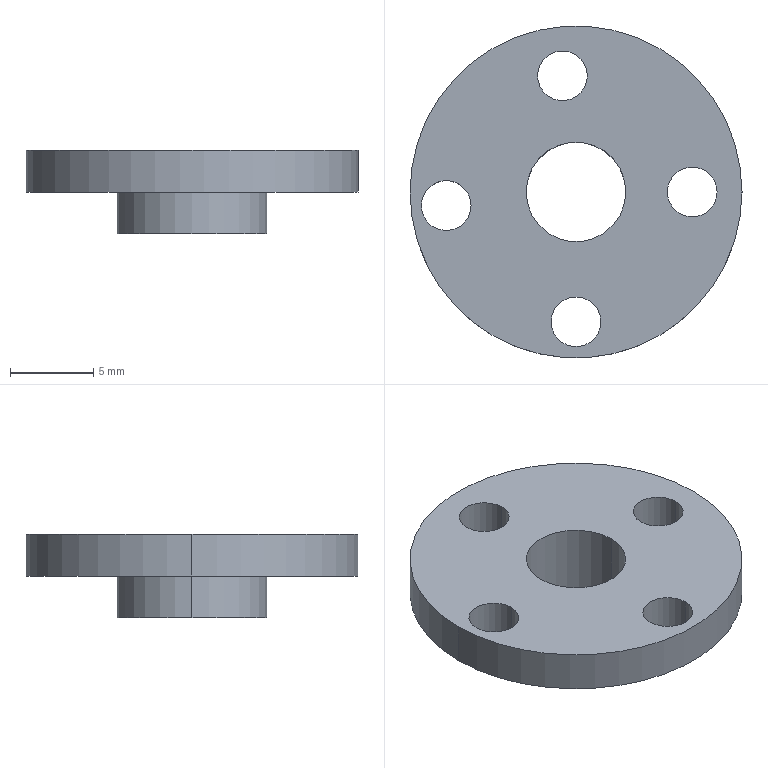Part | SolidWorks | features Cut 1, Extrusion 1, ICE 1 | 1 solid | 17 faces | box 20 x 20 x 5 mm | volume 732.384 mm3 | cylinder 14 | plane 3 | commonest cylinder face diameters 3 x8 6 x2 9 x2 20 x2
STEP:
#1=CARTESIAN_POINT('',(-9.318,-0.8181,2.5));
#2=VERTEX_POINT('',#1);
#3=CARTESIAN_POINT('',(-6.318,-0.8181,2.5));
#4=VERTEX_POINT('',#3);
#5=CARTESIAN_POINT('',(-7.818,-0.8181,2.5));
#6=DIRECTION('',(0.,0.,1.));
#7=DIRECTION('',(1.,0.,0.));
#8=AXIS2_PLACEMENT_3D('',#5,#6,#7);
#9=CIRCLE('',#8,1.5);
#10=EDGE_CURVE('',#2,#4,#9,.T.);
#11=ORIENTED_EDGE('',*,*,#10,.F.);
#12=CARTESIAN_POINT('',(-9.318,-0.8181,5.));
#13=VERTEX_POINT('',#12);
#14=CARTESIAN_POINT('',(-9.318,-0.8181,0.));
#15=DIRECTION('',(0.,0.,1.));
#16=VECTOR('',#15,1000.);
#17=LINE('',#14,#16);
#18=EDGE_CURVE('',#2,#13,#17,.T.);
#19=ORIENTED_EDGE('',*,*,#18,.T.);
#20=CARTESIAN_POINT('',(-6.318,-0.8181,5.));
#21=VERTEX_POINT('',#20);
#22=CARTESIAN_POINT('',(-7.818,-0.8181,5.));
#23=DIRECTION('',(0.,0.,1.));
#24=DIRECTION('',(1.,0.,0.));
#25=AXIS2_PLACEMENT_3D('',#22,#23,#24);
#26=CIRCLE('',#25,1.5);
#27=EDGE_CURVE('',#13,#21,#26,.T.);
#28=ORIENTED_EDGE('',*,*,#27,.T.);
#29=CARTESIAN_POINT('',(-6.318,-0.8181,0.));
#30=DIRECTION('',(0.,0.,1.));
#31=VECTOR('',#30,1000.);
#32=LINE('',#29,#31);
#33=EDGE_CURVE('',#4,#21,#32,.T.);
#34=ORIENTED_EDGE('',*,*,#33,.F.);
#35=EDGE_LOOP('',(#11,#19,#28,#34));
#36=FACE_OUTER_BOUND('',#35,.T.);
#37=CARTESIAN_POINT('',(-7.818,-0.8181,0.));
#38=DIRECTION('',(0.,0.,1.));
#39=DIRECTION('',(1.,0.,0.));
#40=AXIS2_PLACEMENT_3D('',#37,#38,#39);
#41=CYLINDRICAL_SURFACE('',#40,1.5);
#42=ADVANCED_FACE('',(#36),#41,.F.);
#43=CARTESIAN_POINT('',(-1.5,-7.818,2.5));
#44=VERTEX_POINT('',#43);
#45=CARTESIAN_POINT('',(1.5,-7.818,2.5));
#46=VERTEX_POINT('',#45);
#47=CARTESIAN_POINT('',(0.,-7.818,2.5));
#48=DIRECTION('',(0.,0.,1.));
#49=DIRECTION('',(1.,0.,0.));
#50=AXIS2_PLACEMENT_3D('',#47,#48,#49);
#51=CIRCLE('',#50,1.5);
#52=EDGE_CURVE('',#44,#46,#51,.T.);
#53=ORIENTED_EDGE('',*,*,#52,.F.);
#54=CARTESIAN_POINT('',(-1.5,-7.818,5.));
#55=VERTEX_POINT('',#54);
#56=CARTESIAN_POINT('',(-1.5,-7.818,0.));
#57=DIRECTION('',(0.,0.,1.));
#58=VECTOR('',#57,1000.);
#59=LINE('',#56,#58);
#60=EDGE_CURVE('',#44,#55,#59,.T.);
#61=ORIENTED_EDGE('',*,*,#60,.T.);
#62=CARTESIAN_POINT('',(1.5,-7.818,5.));
#63=VERTEX_POINT('',#62);
#64=CARTESIAN_POINT('',(0.,-7.818,5.));
#65=DIRECTION('',(0.,0.,1.));
#66=DIRECTION('',(1.,0.,0.));
#67=AXIS2_PLACEMENT_3D('',#64,#65,#66);
#68=CIRCLE('',#67,1.5);
#69=EDGE_CURVE('',#55,#63,#68,.T.);
#70=ORIENTED_EDGE('',*,*,#69,.T.);
#71=CARTESIAN_POINT('',(1.5,-7.818,0.));
#72=DIRECTION('',(0.,0.,1.));
#73=VECTOR('',#72,1000.);
#74=LINE('',#71,#73);
#75=EDGE_CURVE('',#46,#63,#74,.T.);
#76=ORIENTED_EDGE('',*,*,#75,.F.);
#77=EDGE_LOOP('',(#53,#61,#70,#76));
#78=FACE_OUTER_BOUND('',#77,.T.);
#79=CARTESIAN_POINT('',(0.,-7.818,0.));
#80=DIRECTION('',(0.,0.,1.));
#81=DIRECTION('',(1.,0.,0.));
#82=AXIS2_PLACEMENT_3D('',#79,#80,#81);
#83=CYLINDRICAL_SURFACE('',#82,1.5);
#84=ADVANCED_FACE('',(#78),#83,.F.);
#85=CARTESIAN_POINT('',(5.5,0.,2.5));
#86=VERTEX_POINT('',#85);
#87=CARTESIAN_POINT('',(8.5,0.,2.5));
#88=VERTEX_POINT('',#87);
#89=CARTESIAN_POINT('',(7.,0.,2.5));
#90=DIRECTION('',(0.,0.,1.));
#91=DIRECTION('',(1.,0.,0.));
#92=AXIS2_PLACEMENT_3D('',#89,#90,#91);
#93=CIRCLE('',#92,1.5);
#94=EDGE_CURVE('',#86,#88,#93,.T.);
#95=ORIENTED_EDGE('',*,*,#94,.F.);
#96=CARTESIAN_POINT('',(5.5,0.,5.));
#97=VERTEX_POINT('',#96);
#98=CARTESIAN_POINT('',(5.5,0.,0.));
#99=DIRECTION('',(0.,0.,1.));
#100=VECTOR('',#99,1000.);
#101=LINE('',#98,#100);
#102=EDGE_CURVE('',#86,#97,#101,.T.);
#103=ORIENTED_EDGE('',*,*,#102,.T.);
#104=CARTESIAN_POINT('',(8.5,0.,5.));
#105=VERTEX_POINT('',#104);
#106=CARTESIAN_POINT('',(7.,0.,5.));
#107=DIRECTION('',(0.,0.,1.));
#108=DIRECTION('',(1.,0.,0.));
#109=AXIS2_PLACEMENT_3D('',#106,#107,#108);
#110=CIRCLE('',#109,1.5);
#111=EDGE_CURVE('',#97,#105,#110,.T.);
#112=ORIENTED_EDGE('',*,*,#111,.T.);
#113=CARTESIAN_POINT('',(8.5,0.,0.));
#114=DIRECTION('',(0.,0.,1.));
#115=VECTOR('',#114,1000.);
#116=LINE('',#113,#115);
#117=EDGE_CURVE('',#88,#105,#116,.T.);
#118=ORIENTED_EDGE('',*,*,#117,.F.);
#119=EDGE_LOOP('',(#95,#103,#112,#118));
#120=FACE_OUTER_BOUND('',#119,.T.);
#121=CARTESIAN_POINT('',(7.,0.,0.));
#122=DIRECTION('',(0.,0.,1.));
#123=DIRECTION('',(1.,0.,0.));
#124=AXIS2_PLACEMENT_3D('',#121,#122,#123);
#125=CYLINDRICAL_SURFACE('',#124,1.5);
#126=ADVANCED_FACE('',(#120),#125,.F.);
#127=CARTESIAN_POINT('',(-2.318,7.,2.5));
#128=VERTEX_POINT('',#127);
#129=CARTESIAN_POINT('',(0.6819,7.,2.5));
#130=VERTEX_POINT('',#129);
#131=CARTESIAN_POINT('',(-0.8181,7.,2.5));
#132=DIRECTION('',(0.,0.,1.));
#133=DIRECTION('',(1.,0.,0.));
#134=AXIS2_PLACEMENT_3D('',#131,#132,#133);
#135=CIRCLE('',#134,1.5);
#136=EDGE_CURVE('',#128,#130,#135,.T.);
#137=ORIENTED_EDGE('',*,*,#136,.F.);
#138=CARTESIAN_POINT('',(-2.318,7.,5.));
#139=VERTEX_POINT('',#138);
#140=CARTESIAN_POINT('',(-2.318,7.,0.));
#141=DIRECTION('',(0.,0.,1.));
#142=VECTOR('',#141,1000.);
#143=LINE('',#140,#142);
#144=EDGE_CURVE('',#128,#139,#143,.T.);
#145=ORIENTED_EDGE('',*,*,#144,.T.);
#146=CARTESIAN_POINT('',(0.6819,7.,5.));
#147=VERTEX_POINT('',#146);
#148=CARTESIAN_POINT('',(-0.8181,7.,5.));
#149=DIRECTION('',(0.,0.,1.));
#150=DIRECTION('',(1.,0.,0.));
#151=AXIS2_PLACEMENT_3D('',#148,#149,#150);
#152=CIRCLE('',#151,1.5);
#153=EDGE_CURVE('',#139,#147,#152,.T.);
#154=ORIENTED_EDGE('',*,*,#153,.T.);
#155=CARTESIAN_POINT('',(0.6819,7.,0.));
#156=DIRECTION('',(0.,0.,1.));
#157=VECTOR('',#156,1000.);
#158=LINE('',#155,#157);
#159=EDGE_CURVE('',#130,#147,#158,.T.);
#160=ORIENTED_EDGE('',*,*,#159,.F.);
#161=EDGE_LOOP('',(#137,#145,#154,#160));
#162=FACE_OUTER_BOUND('',#161,.T.);
#163=CARTESIAN_POINT('',(-0.8181,7.,0.));
#164=DIRECTION('',(0.,0.,1.));
#165=DIRECTION('',(1.,0.,0.));
#166=AXIS2_PLACEMENT_3D('',#163,#164,#165);
#167=CYLINDRICAL_SURFACE('',#166,1.5);
#168=ADVANCED_FACE('',(#162),#167,.F.);
#169=CARTESIAN_POINT('',(10.,0.,2.5));
#170=VERTEX_POINT('',#169);
#171=CARTESIAN_POINT('',(-10.,0.,2.5));
#172=VERTEX_POINT('',#171);
#173=CARTESIAN_POINT('',(0.,0.,2.5));
#174=DIRECTION('',(0.,0.,1.));
#175=DIRECTION('',(1.,0.,0.));
#176=AXIS2_PLACEMENT_3D('',#173,#174,#175);
#177=CIRCLE('',#176,10.);
#178=EDGE_CURVE('',#170,#172,#177,.T.);
#179=ORIENTED_EDGE('',*,*,#178,.T.);
#180=CARTESIAN_POINT('',(-10.,0.,5.));
#181=VERTEX_POINT('',#180);
#182=CARTESIAN_POINT('',(-10.,0.,2.5));
#183=DIRECTION('',(0.,0.,1.));
#184=VECTOR('',#183,1000.);
#185=LINE('',#182,#184);
#186=EDGE_CURVE('',#172,#181,#185,.T.);
#187=ORIENTED_EDGE('',*,*,#186,.T.);
#188=CARTESIAN_POINT('',(10.,0.,5.));
#189=VERTEX_POINT('',#188);
#190=CARTESIAN_POINT('',(0.,0.,5.));
#191=DIRECTION('',(0.,0.,1.));
#192=DIRECTION('',(1.,0.,0.));
#193=AXIS2_PLACEMENT_3D('',#190,#191,#192);
#194=CIRCLE('',#193,10.);
#195=EDGE_CURVE('',#189,#181,#194,.T.);
#196=ORIENTED_EDGE('',*,*,#195,.F.);
#197=CARTESIAN_POINT('',(10.,0.,2.5));
#198=DIRECTION('',(0.,0.,1.));
#199=VECTOR('',#198,1000.);
#200=LINE('',#197,#199);
#201=EDGE_CURVE('',#170,#189,#200,.T.);
#202=ORIENTED_EDGE('',*,*,#201,.F.);
#203=EDGE_LOOP('',(#179,#187,#196,#202));
#204=FACE_OUTER_BOUND('',#203,.T.);
#205=CARTESIAN_POINT('',(0.,0.,2.5));
#206=DIRECTION('',(0.,0.,1.));
#207=DIRECTION('',(1.,0.,0.));
#208=AXIS2_PLACEMENT_3D('',#205,#206,#207);
#209=CYLINDRICAL_SURFACE('',#208,10.);
#210=ADVANCED_FACE('',(#204),#209,.T.);
#211=CARTESIAN_POINT('',(-3.,0.,5.));
#212=VERTEX_POINT('',#211);
#213=CARTESIAN_POINT('',(3.,0.,5.));
#214=VERTEX_POINT('',#213);
#215=CARTESIAN_POINT('',(0.,0.,5.));
#216=DIRECTION('',(0.,0.,1.));
#217=DIRECTION('',(1.,0.,0.));
#218=AXIS2_PLACEMENT_3D('',#215,#216,#217);
#219=CIRCLE('',#218,3.);
#220=EDGE_CURVE('',#212,#214,#219,.T.);
#221=ORIENTED_EDGE('',*,*,#220,.T.);
#222=CARTESIAN_POINT('',(3.,0.,0.));
#223=VERTEX_POINT('',#222);
#224=CARTESIAN_POINT('',(3.,0.,3.));
#225=DIRECTION('',(0.,0.,-1.));
#226=VECTOR('',#225,1000.);
#227=LINE('',#224,#226);
#228=EDGE_CURVE('',#214,#223,#227,.T.);
#229=ORIENTED_EDGE('',*,*,#228,.T.);
#230=CARTESIAN_POINT('',(-3.,0.,0.));
#231=VERTEX_POINT('',#230);
#232=CARTESIAN_POINT('',(0.,0.,0.));
#233=DIRECTION('',(0.,0.,1.));
#234=DIRECTION('',(1.,0.,0.));
#235=AXIS2_PLACEMENT_3D('',#232,#233,#234);
#236=CIRCLE('',#235,3.);
#237=EDGE_CURVE('',#231,#223,#236,.T.);
#238=ORIENTED_EDGE('',*,*,#237,.F.);
#239=CARTESIAN_POINT('',(-3.,0.,3.));
#240=DIRECTION('',(0.,0.,-1.));
#241=VECTOR('',#240,1000.);
#242=LINE('',#239,#241);
#243=EDGE_CURVE('',#212,#231,#242,.T.);
#244=ORIENTED_EDGE('',*,*,#243,.F.);
#245=EDGE_LOOP('',(#221,#229,#238,#244));
#246=FACE_OUTER_BOUND('',#245,.T.);
#247=CARTESIAN_POINT('',(0.,0.,3.));
#248=DIRECTION('',(0.,0.,-1.));
#249=DIRECTION('',(-1.,0.,0.));
#250=AXIS2_PLACEMENT_3D('',#247,#248,#249);
#251=CYLINDRICAL_SURFACE('',#250,3.);
#252=ADVANCED_FACE('',(#246),#251,.F.);
#253=CARTESIAN_POINT('',(4.5,0.,2.5));
#254=VERTEX_POINT('',#253);
#255=CARTESIAN_POINT('',(-4.5,0.,2.5));
#256=VERTEX_POINT('',#255);
#257=CARTESIAN_POINT('',(0.,0.,2.5));
#258=DIRECTION('',(0.,0.,1.));
#259=DIRECTION('',(1.,0.,0.));
#260=AXIS2_PLACEMENT_3D('',#257,#258,#259);
#261=CIRCLE('',#260,4.5);
#262=EDGE_CURVE('',#254,#256,#261,.T.);
#263=ORIENTED_EDGE('',*,*,#262,.F.);
#264=CARTESIAN_POINT('',(4.5,0.,0.));
#265=VERTEX_POINT('',#264);
#266=CARTESIAN_POINT('',(4.5,0.,3.));
#267=DIRECTION('',(0.,0.,-1.));
#268=VECTOR('',#267,1000.);
#269=LINE('',#266,#268);
#270=EDGE_CURVE('',#254,#265,#269,.T.);
#271=ORIENTED_EDGE('',*,*,#270,.T.);
#272=CARTESIAN_POINT('',(-4.5,0.,0.));
#273=VERTEX_POINT('',#272);
#274=CARTESIAN_POINT('',(0.,0.,0.));
#275=DIRECTION('',(0.,0.,1.));
#276=DIRECTION('',(1.,0.,0.));
#277=AXIS2_PLACEMENT_3D('',#274,#275,#276);
#278=CIRCLE('',#277,4.5);
#279=EDGE_CURVE('',#265,#273,#278,.T.);
#280=ORIENTED_EDGE('',*,*,#279,.T.);
#281=CARTESIAN_POINT('',(-4.5,0.,3.));
#282=DIRECTION('',(0.,0.,-1.));
#283=VECTOR('',#282,1000.);
#284=LINE('',#281,#283);
#285=EDGE_CURVE('',#256,#273,#284,.T.);
#286=ORIENTED_EDGE('',*,*,#285,.F.);
#287=EDGE_LOOP('',(#263,#271,#280,#286));
#288=FACE_OUTER_BOUND('',#287,.T.);
#289=CARTESIAN_POINT('',(0.,0.,3.));
#290=DIRECTION('',(0.,0.,-1.));
#291=DIRECTION('',(-1.,0.,0.));
#292=AXIS2_PLACEMENT_3D('',#289,#290,#291);
#293=CYLINDRICAL_SURFACE('',#292,4.5);
#294=ADVANCED_FACE('',(#288),#293,.T.);
#295=ORIENTED_EDGE('',*,*,#270,.F.);
#296=CARTESIAN_POINT('',(0.,0.,2.5));
#297=DIRECTION('',(0.,0.,1.));
#298=DIRECTION('',(1.,0.,0.));
#299=AXIS2_PLACEMENT_3D('',#296,#297,#298);
#300=CIRCLE('',#299,4.5);
#301=EDGE_CURVE('',#256,#254,#300,.T.);
#302=ORIENTED_EDGE('',*,*,#301,.F.);
#303=ORIENTED_EDGE('',*,*,#285,.T.);
#304=CARTESIAN_POINT('',(0.,0.,0.));
#305=DIRECTION('',(0.,0.,1.));
#306=DIRECTION('',(1.,0.,0.));
#307=AXIS2_PLACEMENT_3D('',#304,#305,#306);
#308=CIRCLE('',#307,4.5);
#309=EDGE_CURVE('',#273,#265,#308,.T.);
#310=ORIENTED_EDGE('',*,*,#309,.T.);
#311=EDGE_LOOP('',(#295,#302,#303,#310));
#312=FACE_OUTER_BOUND('',#311,.T.);
#313=CARTESIAN_POINT('',(0.,0.,3.));
#314=DIRECTION('',(0.,0.,-1.));
#315=DIRECTION('',(-1.,0.,0.));
#316=AXIS2_PLACEMENT_3D('',#313,#314,#315);
#317=CYLINDRICAL_SURFACE('',#316,4.5);
#318=ADVANCED_FACE('',(#312),#317,.T.);
#319=ORIENTED_EDGE('',*,*,#309,.F.);
#320=ORIENTED_EDGE('',*,*,#279,.F.);
#321=EDGE_LOOP('',(#319,#320));
#322=FACE_OUTER_BOUND('',#321,.T.);
#323=ORIENTED_EDGE('',*,*,#237,.T.);
#324=CARTESIAN_POINT('',(0.,0.,0.));
#325=DIRECTION('',(0.,0.,1.));
#326=DIRECTION('',(1.,0.,0.));
#327=AXIS2_PLACEMENT_3D('',#324,#325,#326);
#328=CIRCLE('',#327,3.);
#329=EDGE_CURVE('',#223,#231,#328,.T.);
#330=ORIENTED_EDGE('',*,*,#329,.T.);
#331=EDGE_LOOP('',(#323,#330));
#332=FACE_BOUND('',#331,.T.);
#333=CARTESIAN_POINT('',(0.,0.,0.));
#334=DIRECTION('',(0.,0.,1.));
#335=DIRECTION('',(1.,0.,0.));
#336=AXIS2_PLACEMENT_3D('',#333,#334,#335);
#337=PLANE('',#336);
#338=ADVANCED_FACE('',(#322,#332),#337,.F.);
#339=ORIENTED_EDGE('',*,*,#228,.F.);
#340=CARTESIAN_POINT('',(0.,0.,5.));
#341=DIRECTION('',(0.,0.,1.));
#342=DIRECTION('',(1.,0.,0.));
#343=AXIS2_PLACEMENT_3D('',#340,#341,#342);
#344=CIRCLE('',#343,3.);
#345=EDGE_CURVE('',#214,#212,#344,.T.);
#346=ORIENTED_EDGE('',*,*,#345,.T.);
#347=ORIENTED_EDGE('',*,*,#243,.T.);
#348=ORIENTED_EDGE('',*,*,#329,.F.);
#349=EDGE_LOOP('',(#339,#346,#347,#348));
#350=FACE_OUTER_BOUND('',#349,.T.);
#351=CARTESIAN_POINT('',(0.,0.,3.));
#352=DIRECTION('',(0.,0.,-1.));
#353=DIRECTION('',(-1.,0.,0.));
#354=AXIS2_PLACEMENT_3D('',#351,#352,#353);
#355=CYLINDRICAL_SURFACE('',#354,3.);
#356=ADVANCED_FACE('',(#350),#355,.F.);
#357=CARTESIAN_POINT('',(-7.818,-0.8181,2.5));
#358=DIRECTION('',(0.,0.,1.));
#359=DIRECTION('',(1.,0.,0.));
#360=AXIS2_PLACEMENT_3D('',#357,#358,#359);
#361=CIRCLE('',#360,1.5);
#362=EDGE_CURVE('',#4,#2,#361,.T.);
#363=ORIENTED_EDGE('',*,*,#362,.T.);
#364=ORIENTED_EDGE('',*,*,#10,.T.);
#365=EDGE_LOOP('',(#363,#364));
#366=FACE_BOUND('',#365,.T.);
#367=CARTESIAN_POINT('',(0.,-7.818,2.5));
#368=DIRECTION('',(0.,0.,1.));
#369=DIRECTION('',(1.,0.,0.));
#370=AXIS2_PLACEMENT_3D('',#367,#368,#369);
#371=CIRCLE('',#370,1.5);
#372=EDGE_CURVE('',#46,#44,#371,.T.);
#373=ORIENTED_EDGE('',*,*,#372,.T.);
#374=ORIENTED_EDGE('',*,*,#52,.T.);
#375=EDGE_LOOP('',(#373,#374));
#376=FACE_BOUND('',#375,.T.);
#377=CARTESIAN_POINT('',(7.,0.,2.5));
#378=DIRECTION('',(0.,0.,1.));
#379=DIRECTION('',(1.,0.,0.));
#380=AXIS2_PLACEMENT_3D('',#377,#378,#379);
#381=CIRCLE('',#380,1.5);
#382=EDGE_CURVE('',#88,#86,#381,.T.);
#383=ORIENTED_EDGE('',*,*,#382,.T.);
#384=ORIENTED_EDGE('',*,*,#94,.T.);
#385=EDGE_LOOP('',(#383,#384));
#386=FACE_BOUND('',#385,.T.);
#387=CARTESIAN_POINT('',(-0.8181,7.,2.5));
#388=DIRECTION('',(0.,0.,1.));
#389=DIRECTION('',(1.,0.,0.));
#390=AXIS2_PLACEMENT_3D('',#387,#388,#389);
#391=CIRCLE('',#390,1.5);
#392=EDGE_CURVE('',#130,#128,#391,.T.);
#393=ORIENTED_EDGE('',*,*,#392,.T.);
#394=ORIENTED_EDGE('',*,*,#136,.T.);
#395=EDGE_LOOP('',(#393,#394));
#396=FACE_BOUND('',#395,.T.);
#397=ORIENTED_EDGE('',*,*,#178,.F.);
#398=CARTESIAN_POINT('',(0.,0.,2.5));
#399=DIRECTION('',(0.,0.,1.));
#400=DIRECTION('',(1.,0.,0.));
#401=AXIS2_PLACEMENT_3D('',#398,#399,#400);
#402=CIRCLE('',#401,10.);
#403=EDGE_CURVE('',#172,#170,#402,.T.);
#404=ORIENTED_EDGE('',*,*,#403,.F.);
#405=EDGE_LOOP('',(#397,#404));
#406=FACE_OUTER_BOUND('',#405,.T.);
#407=ORIENTED_EDGE('',*,*,#301,.T.);
#408=ORIENTED_EDGE('',*,*,#262,.T.);
#409=EDGE_LOOP('',(#407,#408));
#410=FACE_BOUND('',#409,.T.);
#411=CARTESIAN_POINT('',(0.,0.,2.5));
#412=DIRECTION('',(0.,0.,1.));
#413=DIRECTION('',(1.,0.,0.));
#414=AXIS2_PLACEMENT_3D('',#411,#412,#413);
#415=PLANE('',#414);
#416=ADVANCED_FACE('',(#366,#376,#386,#396,#406,#410),#415,.F.);
#417=ORIENTED_EDGE('',*,*,#186,.F.);
#418=ORIENTED_EDGE('',*,*,#403,.T.);
#419=ORIENTED_EDGE('',*,*,#201,.T.);
#420=CARTESIAN_POINT('',(0.,0.,5.));
#421=DIRECTION('',(0.,0.,1.));
#422=DIRECTION('',(1.,0.,0.));
#423=AXIS2_PLACEMENT_3D('',#420,#421,#422);
#424=CIRCLE('',#423,10.);
#425=EDGE_CURVE('',#181,#189,#424,.T.);
#426=ORIENTED_EDGE('',*,*,#425,.F.);
#427=EDGE_LOOP('',(#417,#418,#419,#426));
#428=FACE_OUTER_BOUND('',#427,.T.);
#429=CARTESIAN_POINT('',(0.,0.,2.5));
#430=DIRECTION('',(0.,0.,1.));
#431=DIRECTION('',(1.,0.,0.));
#432=AXIS2_PLACEMENT_3D('',#429,#430,#431);
#433=CYLINDRICAL_SURFACE('',#432,10.);
#434=ADVANCED_FACE('',(#428),#433,.T.);
#435=CARTESIAN_POINT('',(-7.818,-0.8181,5.));
#436=DIRECTION('',(0.,0.,1.));
#437=DIRECTION('',(1.,0.,0.));
#438=AXIS2_PLACEMENT_3D('',#435,#436,#437);
#439=CIRCLE('',#438,1.5);
#440=EDGE_CURVE('',#21,#13,#439,.T.);
#441=ORIENTED_EDGE('',*,*,#440,.F.);
#442=ORIENTED_EDGE('',*,*,#27,.F.);
#443=EDGE_LOOP('',(#441,#442));
#444=FACE_BOUND('',#443,.T.);
#445=CARTESIAN_POINT('',(0.,-7.818,5.));
#446=DIRECTION('',(0.,0.,1.));
#447=DIRECTION('',(1.,0.,0.));
#448=AXIS2_PLACEMENT_3D('',#445,#446,#447);
#449=CIRCLE('',#448,1.5);
#450=EDGE_CURVE('',#63,#55,#449,.T.);
#451=ORIENTED_EDGE('',*,*,#450,.F.);
#452=ORIENTED_EDGE('',*,*,#69,.F.);
#453=EDGE_LOOP('',(#451,#452));
#454=FACE_BOUND('',#453,.T.);
#455=CARTESIAN_POINT('',(7.,0.,5.));
#456=DIRECTION('',(0.,0.,1.));
#457=DIRECTION('',(1.,0.,0.));
#458=AXIS2_PLACEMENT_3D('',#455,#456,#457);
#459=CIRCLE('',#458,1.5);
#460=EDGE_CURVE('',#105,#97,#459,.T.);
#461=ORIENTED_EDGE('',*,*,#460,.F.);
#462=ORIENTED_EDGE('',*,*,#111,.F.);
#463=EDGE_LOOP('',(#461,#462));
#464=FACE_BOUND('',#463,.T.);
#465=CARTESIAN_POINT('',(-0.8181,7.,5.));
#466=DIRECTION('',(0.,0.,1.));
#467=DIRECTION('',(1.,0.,0.));
#468=AXIS2_PLACEMENT_3D('',#465,#466,#467);
#469=CIRCLE('',#468,1.5);
#470=EDGE_CURVE('',#147,#139,#469,.T.);
#471=ORIENTED_EDGE('',*,*,#470,.F.);
#472=ORIENTED_EDGE('',*,*,#153,.F.);
#473=EDGE_LOOP('',(#471,#472));
#474=FACE_BOUND('',#473,.T.);
#475=ORIENTED_EDGE('',*,*,#195,.T.);
#476=ORIENTED_EDGE('',*,*,#425,.T.);
#477=EDGE_LOOP('',(#475,#476));
#478=FACE_OUTER_BOUND('',#477,.T.);
#479=ORIENTED_EDGE('',*,*,#220,.F.);
#480=ORIENTED_EDGE('',*,*,#345,.F.);
#481=EDGE_LOOP('',(#479,#480));
#482=FACE_BOUND('',#481,.T.);
#483=CARTESIAN_POINT('',(0.,0.,5.));
#484=DIRECTION('',(0.,0.,1.));
#485=DIRECTION('',(1.,0.,0.));
#486=AXIS2_PLACEMENT_3D('',#483,#484,#485);
#487=PLANE('',#486);
#488=ADVANCED_FACE('',(#444,#454,#464,#474,#478,#482),#487,.T.);
#489=ORIENTED_EDGE('',*,*,#144,.F.);
#490=ORIENTED_EDGE('',*,*,#392,.F.);
#491=ORIENTED_EDGE('',*,*,#159,.T.);
#492=ORIENTED_EDGE('',*,*,#470,.T.);
#493=EDGE_LOOP('',(#489,#490,#491,#492));
#494=FACE_OUTER_BOUND('',#493,.T.);
#495=CARTESIAN_POINT('',(-0.8181,7.,0.));
#496=DIRECTION('',(0.,0.,1.));
#497=DIRECTION('',(1.,0.,0.));
#498=AXIS2_PLACEMENT_3D('',#495,#496,#497);
#499=CYLINDRICAL_SURFACE('',#498,1.5);
#500=ADVANCED_FACE('',(#494),#499,.F.);
#501=ORIENTED_EDGE('',*,*,#102,.F.);
#502=ORIENTED_EDGE('',*,*,#382,.F.);
#503=ORIENTED_EDGE('',*,*,#117,.T.);
#504=ORIENTED_EDGE('',*,*,#460,.T.);
#505=EDGE_LOOP('',(#501,#502,#503,#504));
#506=FACE_OUTER_BOUND('',#505,.T.);
#507=CARTESIAN_POINT('',(7.,0.,0.));
#508=DIRECTION('',(0.,0.,1.));
#509=DIRECTION('',(1.,0.,0.));
#510=AXIS2_PLACEMENT_3D('',#507,#508,#509);
#511=CYLINDRICAL_SURFACE('',#510,1.5);
#512=ADVANCED_FACE('',(#506),#511,.F.);
#513=ORIENTED_EDGE('',*,*,#60,.F.);
#514=ORIENTED_EDGE('',*,*,#372,.F.);
#515=ORIENTED_EDGE('',*,*,#75,.T.);
#516=ORIENTED_EDGE('',*,*,#450,.T.);
#517=EDGE_LOOP('',(#513,#514,#515,#516));
#518=FACE_OUTER_BOUND('',#517,.T.);
#519=CARTESIAN_POINT('',(0.,-7.818,0.));
#520=DIRECTION('',(0.,0.,1.));
#521=DIRECTION('',(1.,0.,0.));
#522=AXIS2_PLACEMENT_3D('',#519,#520,#521);
#523=CYLINDRICAL_SURFACE('',#522,1.5);
#524=ADVANCED_FACE('',(#518),#523,.F.);
#525=ORIENTED_EDGE('',*,*,#18,.F.);
#526=ORIENTED_EDGE('',*,*,#362,.F.);
#527=ORIENTED_EDGE('',*,*,#33,.T.);
#528=ORIENTED_EDGE('',*,*,#440,.T.);
#529=EDGE_LOOP('',(#525,#526,#527,#528));
#530=FACE_OUTER_BOUND('',#529,.T.);
#531=CARTESIAN_POINT('',(-7.818,-0.8181,0.));
#532=DIRECTION('',(0.,0.,1.));
#533=DIRECTION('',(1.,0.,0.));
#534=AXIS2_PLACEMENT_3D('',#531,#532,#533);
#535=CYLINDRICAL_SURFACE('',#534,1.5);
#536=ADVANCED_FACE('',(#530),#535,.F.);
#537=CLOSED_SHELL('',(#42,#84,#126,#168,#210,#252,#294,#318,#338,#356,#416,#434,#488,#500,#512,#524,#536));
#538=MANIFOLD_SOLID_BREP('',#537);
#539=CARTESIAN_POINT('',(0.,0.,0.));
#540=DIRECTION('',(0.,0.,1.));
#541=DIRECTION('',(1.,0.,0.));
#542=AXIS2_PLACEMENT_3D('',#539,#540,#541);
#543=(LENGTH_UNIT()NAMED_UNIT(*)SI_UNIT(.MILLI.,.METRE.));
#544=UNCERTAINTY_MEASURE_WITH_UNIT(LENGTH_MEASURE(0.00001),#543,'','');
#545=(NAMED_UNIT(*)PLANE_ANGLE_UNIT()SI_UNIT($,.RADIAN.));
#546=(NAMED_UNIT(*)SI_UNIT($,.STERADIAN.)SOLID_ANGLE_UNIT());
#547=(GEOMETRIC_REPRESENTATION_CONTEXT(3)GLOBAL_UNCERTAINTY_ASSIGNED_CONTEXT((#544))GLOBAL_UNIT_ASSIGNED_CONTEXT((#543,#545,#546))REPRESENTATION_CONTEXT('',''));
#548=ADVANCED_BREP_SHAPE_REPRESENTATION('',(#538,#542),#547);